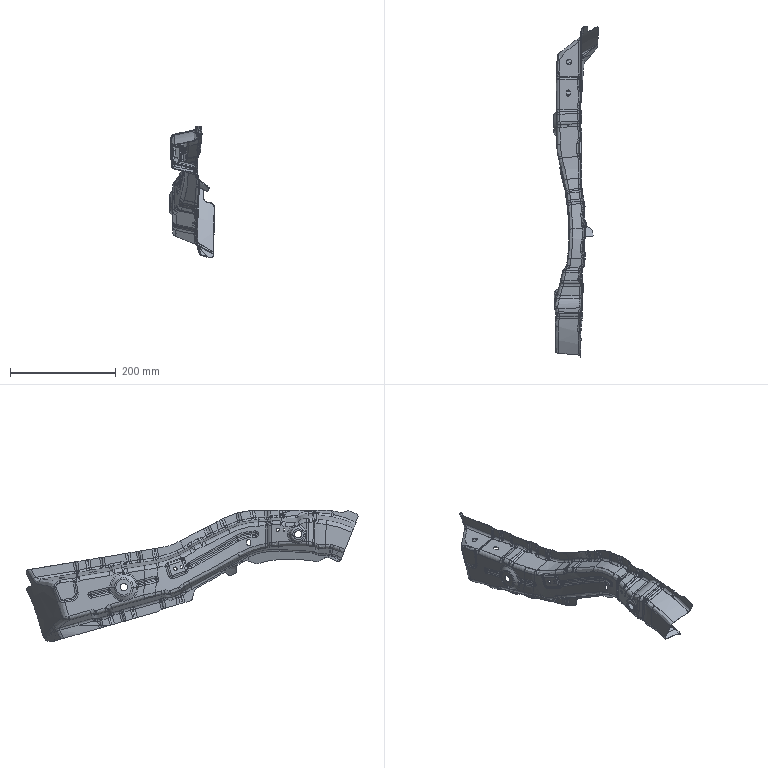Part | 1 solid | 1268 faces | box 84.948 x 628.247 x 248.659 mm | volume 126298 mm3 | spline 878 | cylinder 263 | plane 94 | sphere 28 | torus 4 | other 1 | commonest cylinder face diameters 16 x41 10 x32 13.6 x29 20 x18 12.4 x17 7.6 x13